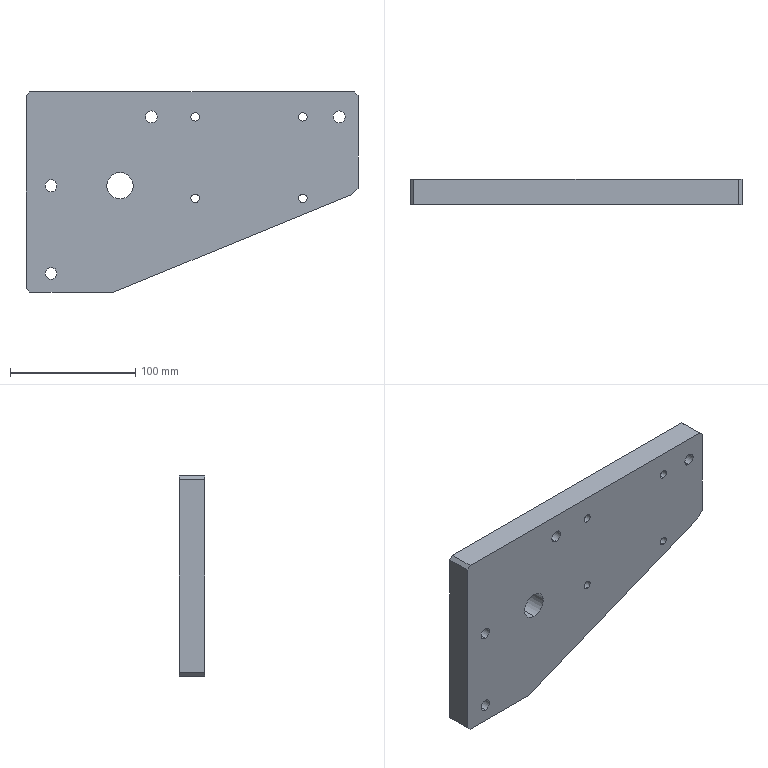Part | STEP file | Caster support plate | 1 solid | 29 faces | box 265 x 20 x 160 mm | volume 676074 mm3 | cylinder 18 | plane 11 | commonest cylinder face diameters 6.8 x8 9.5 x8 21 x2